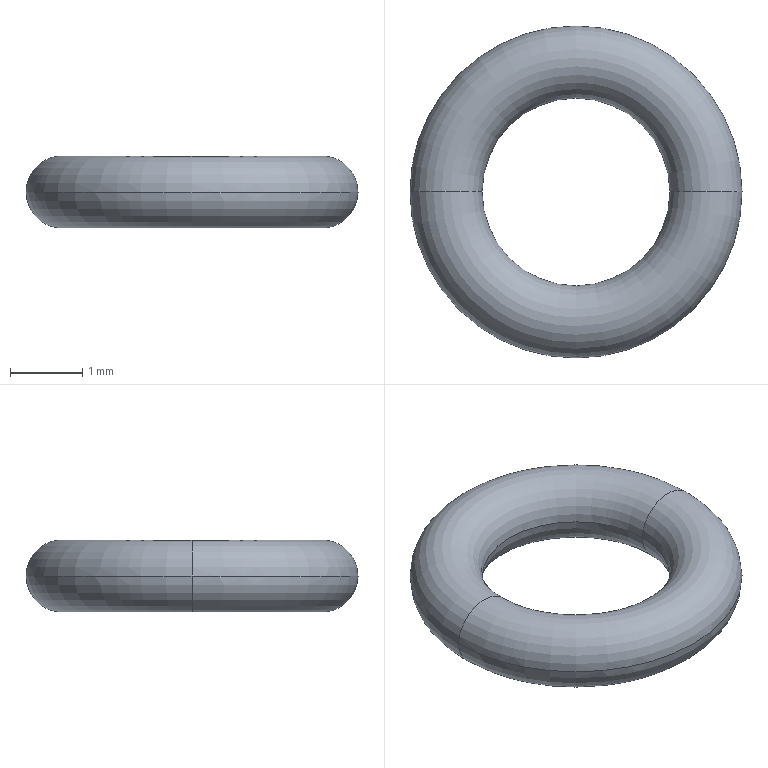Part | SolidWorks | features RefAxis 1, Revolution 1 | 1 solid | 4 faces | box 4.6 x 4.6 x 1 mm | volume 8.883 mm3 | torus 4
STEP:
#1=CARTESIAN_POINT('',(2.3,0.,0.));
#2=VERTEX_POINT('',#1);
#3=CARTESIAN_POINT('',(1.3,0.,0.));
#4=VERTEX_POINT('',#3);
#5=CARTESIAN_POINT('',(1.8,0.,0.));
#6=DIRECTION('',(0.,1.,0.));
#7=DIRECTION('',(-1.,0.,0.));
#8=AXIS2_PLACEMENT_3D('',#5,#6,#7);
#9=CIRCLE('',#8,0.5);
#10=EDGE_CURVE('',#2,#4,#9,.T.);
#11=ORIENTED_EDGE('',*,*,#10,.F.);
#12=CARTESIAN_POINT('',(-2.3,0.,0.));
#13=VERTEX_POINT('',#12);
#14=CARTESIAN_POINT('',(0.,0.,0.));
#15=DIRECTION('',(0.,0.,-1.));
#16=DIRECTION('',(-1.,0.,0.));
#17=AXIS2_PLACEMENT_3D('',#14,#15,#16);
#18=CIRCLE('',#17,2.3);
#19=EDGE_CURVE('',#2,#13,#18,.T.);
#20=ORIENTED_EDGE('',*,*,#19,.T.);
#21=CARTESIAN_POINT('',(-1.3,0.,0.));
#22=VERTEX_POINT('',#21);
#23=CARTESIAN_POINT('',(-1.8,0.,0.));
#24=DIRECTION('',(0.,-1.,0.));
#25=DIRECTION('',(0.,0.,-1.));
#26=AXIS2_PLACEMENT_3D('',#23,#24,#25);
#27=CIRCLE('',#26,0.5);
#28=EDGE_CURVE('',#13,#22,#27,.T.);
#29=ORIENTED_EDGE('',*,*,#28,.T.);
#30=CARTESIAN_POINT('',(0.,0.,0.));
#31=DIRECTION('',(0.,0.,-1.));
#32=DIRECTION('',(-1.,0.,0.));
#33=AXIS2_PLACEMENT_3D('',#30,#31,#32);
#34=CIRCLE('',#33,1.3);
#35=EDGE_CURVE('',#4,#22,#34,.T.);
#36=ORIENTED_EDGE('',*,*,#35,.F.);
#37=EDGE_LOOP('',(#11,#20,#29,#36));
#38=FACE_OUTER_BOUND('',#37,.T.);
#39=CARTESIAN_POINT('',(0.,0.,0.));
#40=DIRECTION('',(0.,0.,-1.));
#41=DIRECTION('',(-1.,0.,0.));
#42=AXIS2_PLACEMENT_3D('',#39,#40,#41);
#43=TOROIDAL_SURFACE('',#42,1.8,0.5);
#44=ADVANCED_FACE('',(#38),#43,.T.);
#45=ORIENTED_EDGE('',*,*,#28,.F.);
#46=CARTESIAN_POINT('',(0.,0.,0.));
#47=DIRECTION('',(0.,0.,-1.));
#48=DIRECTION('',(-1.,0.,0.));
#49=AXIS2_PLACEMENT_3D('',#46,#47,#48);
#50=CIRCLE('',#49,2.3);
#51=EDGE_CURVE('',#13,#2,#50,.T.);
#52=ORIENTED_EDGE('',*,*,#51,.T.);
#53=ORIENTED_EDGE('',*,*,#10,.T.);
#54=CARTESIAN_POINT('',(0.,0.,0.));
#55=DIRECTION('',(0.,0.,-1.));
#56=DIRECTION('',(-1.,0.,0.));
#57=AXIS2_PLACEMENT_3D('',#54,#55,#56);
#58=CIRCLE('',#57,1.3);
#59=EDGE_CURVE('',#22,#4,#58,.T.);
#60=ORIENTED_EDGE('',*,*,#59,.F.);
#61=EDGE_LOOP('',(#45,#52,#53,#60));
#62=FACE_OUTER_BOUND('',#61,.T.);
#63=CARTESIAN_POINT('',(0.,0.,0.));
#64=DIRECTION('',(0.,0.,-1.));
#65=DIRECTION('',(-1.,0.,0.));
#66=AXIS2_PLACEMENT_3D('',#63,#64,#65);
#67=TOROIDAL_SURFACE('',#66,1.8,0.5);
#68=ADVANCED_FACE('',(#62),#67,.T.);
#69=ORIENTED_EDGE('',*,*,#51,.F.);
#70=CARTESIAN_POINT('',(-1.8,0.,0.));
#71=DIRECTION('',(0.,-1.,0.));
#72=DIRECTION('',(0.,0.,-1.));
#73=AXIS2_PLACEMENT_3D('',#70,#71,#72);
#74=CIRCLE('',#73,0.5);
#75=EDGE_CURVE('',#22,#13,#74,.T.);
#76=ORIENTED_EDGE('',*,*,#75,.F.);
#77=ORIENTED_EDGE('',*,*,#59,.T.);
#78=CARTESIAN_POINT('',(1.8,0.,0.));
#79=DIRECTION('',(0.,1.,0.));
#80=DIRECTION('',(-1.,0.,0.));
#81=AXIS2_PLACEMENT_3D('',#78,#79,#80);
#82=CIRCLE('',#81,0.5);
#83=EDGE_CURVE('',#4,#2,#82,.T.);
#84=ORIENTED_EDGE('',*,*,#83,.T.);
#85=EDGE_LOOP('',(#69,#76,#77,#84));
#86=FACE_OUTER_BOUND('',#85,.T.);
#87=CARTESIAN_POINT('',(0.,0.,0.));
#88=DIRECTION('',(0.,0.,-1.));
#89=DIRECTION('',(-1.,0.,0.));
#90=AXIS2_PLACEMENT_3D('',#87,#88,#89);
#91=TOROIDAL_SURFACE('',#90,1.8,0.5);
#92=ADVANCED_FACE('',(#86),#91,.T.);
#93=ORIENTED_EDGE('',*,*,#19,.F.);
#94=ORIENTED_EDGE('',*,*,#83,.F.);
#95=ORIENTED_EDGE('',*,*,#35,.T.);
#96=ORIENTED_EDGE('',*,*,#75,.T.);
#97=EDGE_LOOP('',(#93,#94,#95,#96));
#98=FACE_OUTER_BOUND('',#97,.T.);
#99=CARTESIAN_POINT('',(0.,0.,0.));
#100=DIRECTION('',(0.,0.,-1.));
#101=DIRECTION('',(-1.,0.,0.));
#102=AXIS2_PLACEMENT_3D('',#99,#100,#101);
#103=TOROIDAL_SURFACE('',#102,1.8,0.5);
#104=ADVANCED_FACE('',(#98),#103,.T.);
#105=CLOSED_SHELL('',(#44,#68,#92,#104));
#106=MANIFOLD_SOLID_BREP('',#105);
#107=CARTESIAN_POINT('',(0.,0.,0.));
#108=DIRECTION('',(0.,0.,1.));
#109=DIRECTION('',(1.,0.,0.));
#110=AXIS2_PLACEMENT_3D('',#107,#108,#109);
#111=(LENGTH_UNIT()NAMED_UNIT(*)SI_UNIT(.MILLI.,.METRE.));
#112=UNCERTAINTY_MEASURE_WITH_UNIT(LENGTH_MEASURE(0.00001),#111,'','');
#113=(NAMED_UNIT(*)PLANE_ANGLE_UNIT()SI_UNIT($,.RADIAN.));
#114=(NAMED_UNIT(*)SI_UNIT($,.STERADIAN.)SOLID_ANGLE_UNIT());
#115=(GEOMETRIC_REPRESENTATION_CONTEXT(3)GLOBAL_UNCERTAINTY_ASSIGNED_CONTEXT((#112))GLOBAL_UNIT_ASSIGNED_CONTEXT((#111,#113,#114))REPRESENTATION_CONTEXT('',''));
#116=ADVANCED_BREP_SHAPE_REPRESENTATION('',(#106,#110),#115);